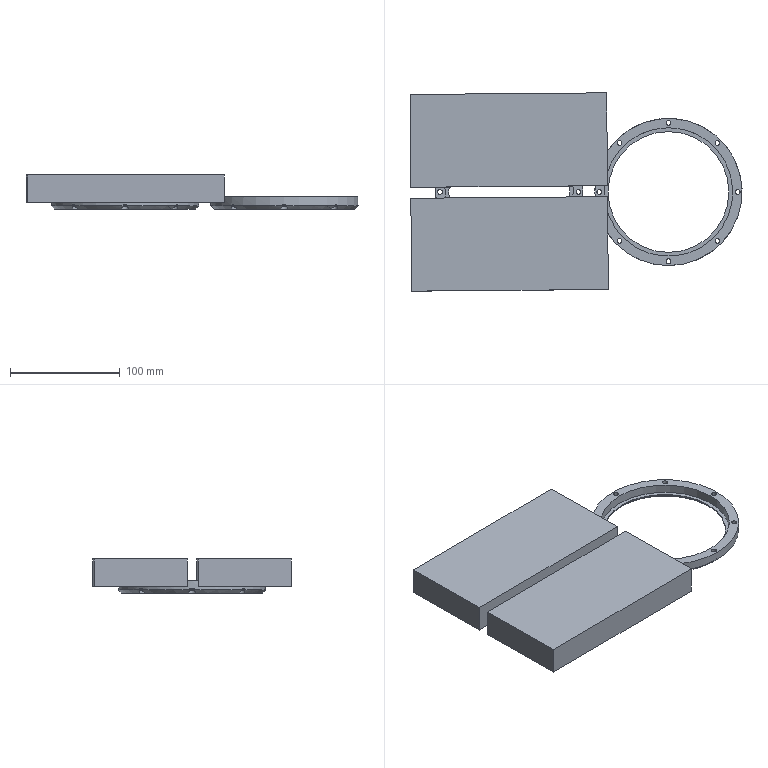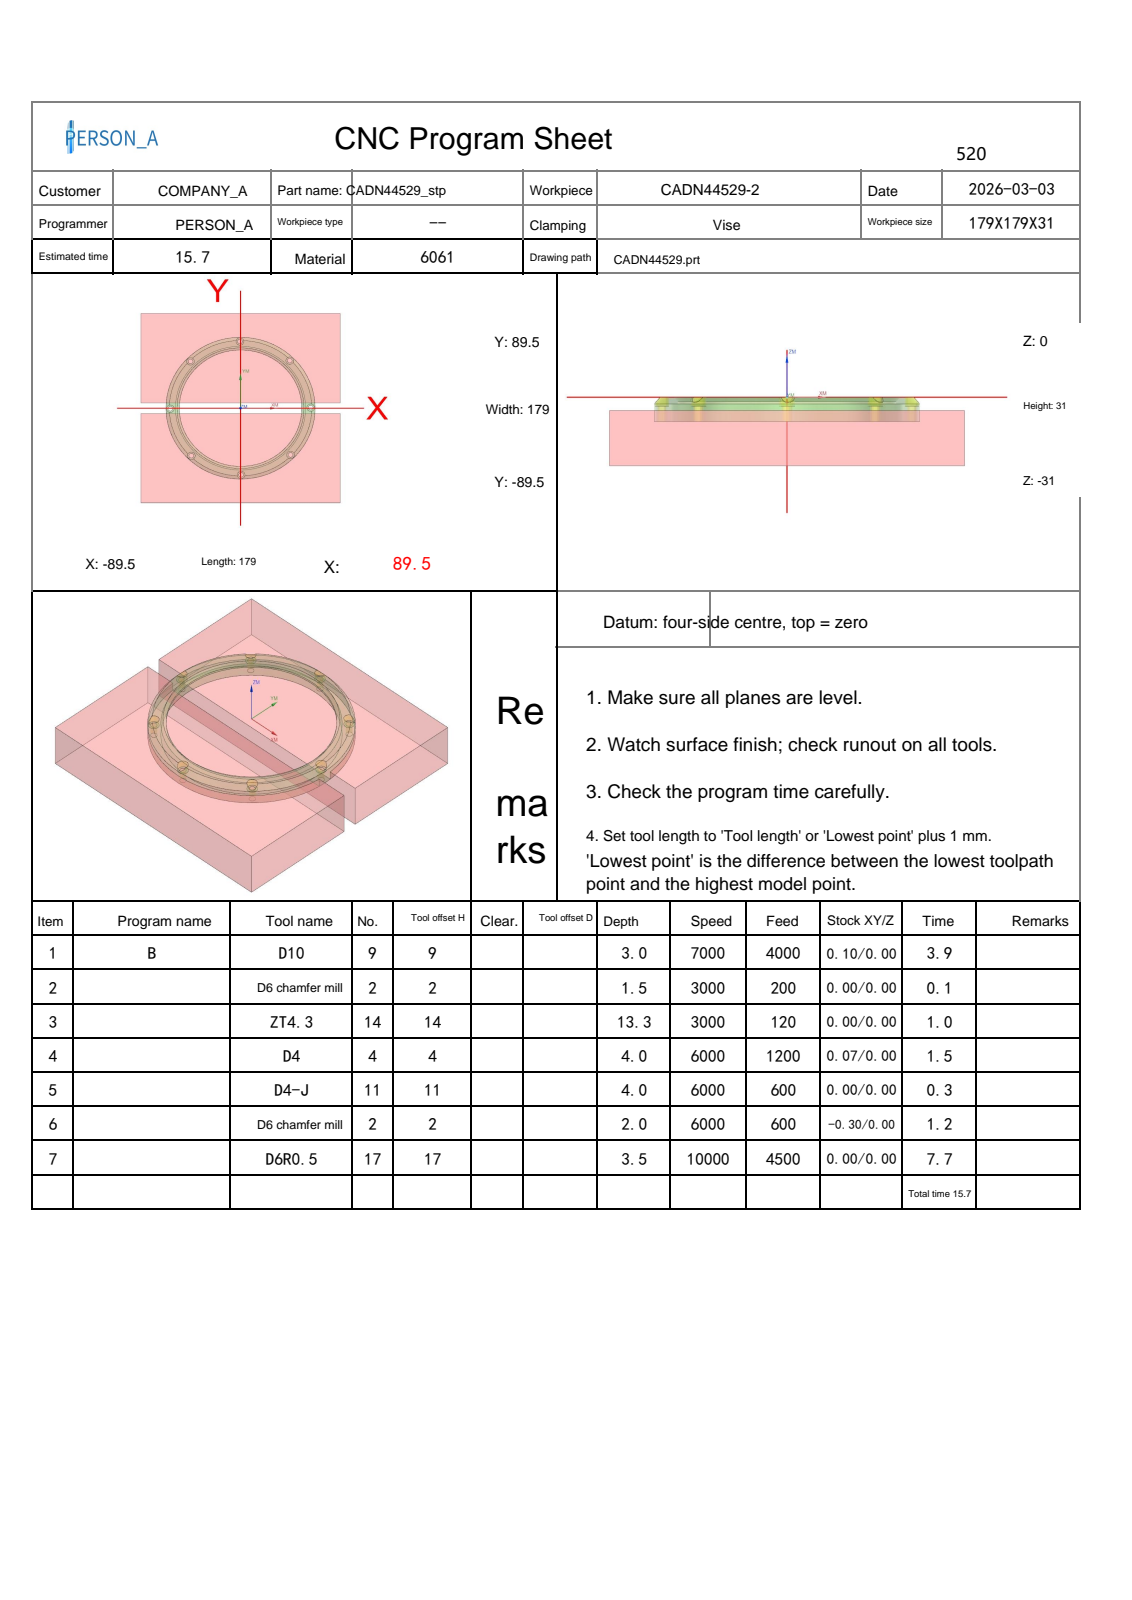NC program | NX | posted by the shop | part box 302.234 x 180.468 x 31 mm
Lines 22986 to 24363 of 75694:
N7 T17 M06
(D6R0.5  D=6. R=0.5 H=17 ce=0.00 di=0.00)
G00 G90 G54 X46.376 Y-28.084 M03 S10000
G43 H17 Z50.
M08
Z1.5
G01 X46.877 Y-27.259 Z1.449 F4500.
X47.6 Y-25.976 Z1.372
X48.553 Y-24.148 Z1.264
X49.436 Y-22.285 Z1.156
X50.247 Y-20.39 Z1.048
X50.986 Y-18.466 Z.94
X51.651 Y-16.515 Z.832
X52.241 Y-14.54 Z.724
X52.756 Y-12.544 Z.616
X53.194 Y-10.53 Z.508
X53.556 Y-8.501 Z.4
X53.84 Y-6.459 Z.292
X54.047 Y-4.408 Z.184
X54.175 Y-2.351 Z.076
X54.226 Y-.29 Z-.032
X54.22 Y.446 Z-.071
G03 X0.0 Y54.221 I-54.22 J-.447
X-54.221 Y-.001 I0.0 J-54.221
X0.0 Y-54.222 I54.221 J0.0
X54.221 Y-.001 I0.0 J54.221
X54.22 Y.446 I-54.221 J0.0
G01 X54.215 Y.814
X54.209 Y1.181
X54.198 Y1.549
X54.188 Y1.916
X54.157 Y2.651
X54.116 Y3.385
X54.064 Y4.119 Z-.072
X54.003 Y4.851
X53.933 Y5.583
X53.852 Y6.314
X53.761 Y7.044
X53.66 Y7.772
X53.55 Y8.499
X53.429 Y9.224 Z-.073
X53.299 Y9.948
X53.159 Y10.67
X53.01 Y11.389
X52.85 Y12.107
X52.681 Y12.823
X52.502 Y13.536 Z-.074
X52.313 Y14.247
X52.115 Y14.955
X51.908 Y15.66
X51.69 Y16.362
X51.463 Y17.062
X51.227 Y17.758
X50.982 Y18.451 Z-.075
X50.726 Y19.14
X50.462 Y19.826
X50.188 Y20.509
X49.906 Y21.187
X49.614 Y21.862
X49.312 Y22.533 Z-.076
X49.002 Y23.199
X48.683 Y23.862
X48.355 Y24.52
X48.018 Y25.173
X47.672 Y25.822
X47.317 Y26.466
X46.954 Y27.105 Z-.077
X46.582 Y27.739
X46.201 Y28.368
X45.812 Y28.992
X45.414 Y29.61
X45.009 Y30.223
X44.594 Y30.831 Z-.078
X44.172 Y31.433
X43.742 Y32.029
X43.303 Y32.619
X42.857 Y33.203
X42.402 Y33.781
X41.94 Y34.353
X41.471 Y34.918 Z-.079
X40.993 Y35.477
X40.508 Y36.03
X40.016 Y36.575
X39.516 Y37.115
X39.009 Y37.647
X38.495 Y38.172 Z-.08
X37.973 Y38.691
X37.445 Y39.202
X36.91 Y39.706
X36.368 Y40.203
X35.819 Y40.692
X35.264 Y41.174
X34.702 Y41.648 Z-.081
X34.134 Y42.115
X33.56 Y42.574
X32.98 Y43.025
X32.393 Y43.468
X31.8 Y43.903
X31.202 Y44.33
X30.598 Y44.749 Z-.082
X29.988 Y45.16
X29.373 Y45.562
X28.752 Y45.956
X28.127 Y46.342
X27.495 Y46.719
X26.859 Y47.087 Z-.083
X26.218 Y47.447
X25.572 Y47.798
X24.922 Y48.14
X24.267 Y48.474
X23.607 Y48.798
X22.943 Y49.114
X22.275 Y49.42 Z-.084
X21.603 Y49.717
X20.926 Y50.006
X20.246 Y50.285
X19.562 Y50.554
X18.875 Y50.815
X18.184 Y51.066 Z-.085
X17.49 Y51.308
X16.793 Y51.54
X16.092 Y51.763
X15.389 Y51.976
X14.682 Y52.18
X13.973 Y52.374
X13.262 Y52.559 Z-.086
X12.548 Y52.734
X11.832 Y52.899
X11.113 Y53.054
X10.393 Y53.2
X9.67 Y53.336
X8.946 Y53.462 Z-.087
X8.22 Y53.578
X7.493 Y53.684
X6.764 Y53.781
X6.034 Y53.868
X5.303 Y53.944
X4.571 Y54.011
X3.838 Y54.068 Z-.088
X3.105 Y54.115
X2.371 Y54.152
X1.636 Y54.179
X.901 Y54.196
X.289 Y54.201
X-.324 Y54.202
X-.446
X-.569 Y54.2 Z-.089
X-1.296 Y54.187
X-2.024 Y54.165
X-2.751 Y54.133
X-3.477 Y54.091
X-4.203 Y54.039
X-4.928 Y53.978
X-5.652 Y53.907 Z-.09
X-6.376 Y53.826
X-7.098 Y53.735
X-7.818 Y53.635
X-8.538 Y53.525
X-9.255 Y53.405
X-9.972 Y53.276
X-10.686 Y53.137 Z-.091
X-11.398 Y52.989
X-12.109 Y52.831
X-12.817 Y52.663
X-13.523 Y52.486
X-14.226 Y52.3
X-14.927 Y52.104 Z-.092
X-15.625 Y51.899
X-16.32 Y51.684
X-17.013 Y51.46
X-17.702 Y51.227
X-18.388 Y50.985
X-19.071 Y50.733
X-19.75 Y50.472 Z-.093
X-20.426 Y50.203
X-21.098 Y49.924
X-21.766 Y49.636
X-22.431 Y49.339
X-23.091 Y49.033
X-23.747 Y48.719 Z-.094
X-24.399 Y48.395
X-25.046 Y48.063
X-25.689 Y47.723
X-26.328 Y47.373
X-26.961 Y47.015
X-27.59 Y46.649
X-28.214 Y46.274 Z-.095
X-28.832 Y45.891
X-29.446 Y45.5
X-30.054 Y45.1
X-30.656 Y44.693
X-31.254 Y44.277
X-31.845 Y43.853
X-32.431 Y43.422 Z-.096
X-33.011 Y42.982
X-33.585 Y42.535
X-34.153 Y42.08
X-34.714 Y41.618
X-35.27 Y41.148
X-35.819 Y40.671 Z-.097
X-36.362 Y40.186
X-36.898 Y39.694
X-37.427 Y39.195
X-37.95 Y38.689
X-38.466 Y38.176
X-38.975 Y37.656
X-39.477 Y37.129 Z-.098
X-39.972 Y36.596
X-40.459 Y36.056
X-40.94 Y35.509
X-41.413 Y34.956
X-41.878 Y34.397
X-42.336 Y33.832
X-42.786 Y33.26 Z-.099
X-43.229 Y32.683
X-43.663 Y32.099
X-44.09 Y31.51
X-44.509 Y30.915
X-44.92 Y30.315
X-45.323 Y29.709 Z-.1
X-45.718 Y29.098
X-46.104 Y28.481
X-46.482 Y27.86
X-46.852 Y27.233
X-47.213 Y26.601
X-47.566 Y25.965
X-47.91 Y25.324 Z-.101
X-48.246 Y24.679
X-48.572 Y24.029
X-48.891 Y23.374
X-49.2 Y22.716
X-49.5 Y22.053
X-49.792 Y21.386 Z-.102
X-50.074 Y20.716
X-50.348 Y20.042
X-50.612 Y19.364
X-50.867 Y18.683
X-51.113 Y17.998
X-51.35 Y17.31
X-51.578 Y16.619 Z-.103
X-51.796 Y15.925
X-52.005 Y15.228
X-52.205 Y14.529
X-52.395 Y13.827
X-52.576 Y13.122
X-52.747 Y12.415
X-52.909 Y11.706 Z-.104
X-53.061 Y10.994
X-53.204 Y10.281
X-53.337 Y9.566
X-53.46 Y8.849
X-53.574 Y8.13
X-53.678 Y7.41 Z-.105
X-53.773 Y6.689
X-53.858 Y5.966
X-53.933 Y5.243
X-53.998 Y4.518
X-54.054 Y3.793
X-54.1 Y3.067
X-54.136 Y2.34 Z-.106
X-54.162 Y1.613
X-54.179 Y.886
X-54.186 Y.158
X-54.183 Y-.569
X-54.17 Y-1.296
X-54.148 Y-2.024 Z-.107
X-54.116 Y-2.75
X-54.074 Y-3.477
X-54.022 Y-4.202
X-53.961 Y-4.927
X-53.89 Y-5.651
X-53.809 Y-6.374
X-53.718 Y-7.096 Z-.108
X-53.618 Y-7.816
X-53.508 Y-8.535
X-53.388 Y-9.253
X-53.259 Y-9.969
X-53.121 Y-10.683
X-52.972 Y-11.395
X-52.814 Y-12.105 Z-.109
X-52.647 Y-12.813
X-52.47 Y-13.519
X-52.284 Y-14.222
X-52.088 Y-14.923
X-51.883 Y-15.62
X-51.668 Y-16.316 Z-.11
X-51.444 Y-17.008
X-51.211 Y-17.697
X-50.969 Y-18.383
X-50.717 Y-19.065
X-50.457 Y-19.744
X-50.187 Y-20.42
X-49.908 Y-21.092 Z-.111
X-49.621 Y-21.76
X-49.324 Y-22.424
X-49.018 Y-23.084
X-48.704 Y-23.74
X-48.381 Y-24.392
X-48.049 Y-25.039
X-47.708 Y-25.682 Z-.112
X-47.359 Y-26.32
X-47.061 Y-26.847
X-46.758 Y-27.37
X-46.696 Y-27.476
X-46.635 Y-27.582
X-46.26 Y-28.205
X-45.877 Y-28.824
X-45.486 Y-29.437 Z-.113
X-45.087 Y-30.045
X-44.679 Y-30.647
X-44.263 Y-31.244
X-43.84 Y-31.835
X-43.408 Y-32.421
X-42.969 Y-33.001
X-42.522 Y-33.575 Z-.114
X-42.067 Y-34.142
X-41.605 Y-34.704
X-41.135 Y-35.259
X-40.658 Y-35.808
X-40.174 Y-36.351
X-39.682 Y-36.887 Z-.115
X-39.183 Y-37.416
X-38.677 Y-37.938
X-38.164 Y-38.454
X-37.644 Y-38.963
X-37.118 Y-39.465
X-36.584 Y-39.959
X-36.044 Y-40.447 Z-.116
X-35.498 Y-40.927
X-34.945 Y-41.4
X-34.386 Y-41.865
X-33.821 Y-42.323
X-33.25 Y-42.773
X-32.672 Y-43.215
X-32.089 Y-43.65 Z-.117
X-31.5 Y-44.076
X-30.906 Y-44.495
X-30.305 Y-44.906
X-29.7 Y-45.309
X-29.089 Y-45.703
X-28.472 Y-46.089 Z-.118
X-27.851 Y-46.467
X-27.224 Y-46.837
X-26.593 Y-47.198
X-25.957 Y-47.551
X-25.316 Y-47.895
X-24.671 Y-48.23
X-24.021 Y-48.557 Z-.119
X-23.367 Y-48.875
X-22.709 Y-49.184
X-22.046 Y-49.484
X-21.38 Y-49.776
X-20.71 Y-50.058
X-20.036 Y-50.331
X-19.358 Y-50.596 Z-.12
X-18.677 Y-50.851
X-17.993 Y-51.097
X-17.305 Y-51.334
X-16.614 Y-51.561
X-15.92 Y-51.779
X-15.224 Y-51.988 Z-.121
X-14.525 Y-52.188
X-13.823 Y-52.378
X-13.118 Y-52.559
X-12.411 Y-52.73
X-11.702 Y-52.892
X-10.991 Y-53.044
X-10.278 Y-53.186 Z-.122
X-9.563 Y-53.319
X-8.846 Y-53.443
X-8.128 Y-53.557
X-7.408 Y-53.661
X-6.687 Y-53.755
X-5.965 Y-53.84 Z-.123
X-5.241 Y-53.915
X-4.879 Y-53.949
X-4.517 Y-53.981
X-4.155 Y-54.01
X-3.792 Y-54.036
X-3.429 Y-54.061
X-3.066 Y-54.082
X-2.703 Y-54.102
X-2.34 Y-54.118
X-1.977 Y-54.133
X-1.613 Y-54.145
X-1.25 Y-54.154
X-.886 Y-54.161 Z-.124
X-.159 Y-54.168
X.568 Y-54.166
X1.295 Y-54.152
X2.022 Y-54.13
X2.386 Y-54.116
X2.749 Y-54.098
X3.112 Y-54.079
X3.475 Y-54.056
X3.838 Y-54.032 Z-.125
X4.2 Y-54.004
X4.563 Y-53.975
X4.925 Y-53.943
X5.287 Y-53.909
X5.649 Y-53.872
X6.01 Y-53.833
X6.371 Y-53.791
X6.732 Y-53.747
X7.093 Y-53.7
X7.453 Y-53.652
X7.813 Y-53.6
X8.173 Y-53.547
X8.532 Y-53.49 Z-.126
X8.891 Y-53.432
X9.249 Y-53.371
X9.607 Y-53.308
X9.965 Y-53.242
X10.322 Y-53.174
X10.679 Y-53.103
X11.035 Y-53.031
X11.391 Y-52.955
X11.746 Y-52.878
X12.101 Y-52.797
X12.455 Y-52.715
X12.808 Y-52.629
X13.161 Y-52.543 Z-.127
X13.514 Y-52.452
X13.866 Y-52.361
X14.216 Y-52.266
X14.567 Y-52.17
X14.917 Y-52.07
X15.266 Y-51.97
X15.615 Y-51.865
X15.963 Y-51.76
X16.309 Y-51.651
X16.656 Y-51.541
X17.001 Y-51.427
X17.346 Y-51.313
X17.69 Y-51.194
X18.034 Y-51.075 Z-.128
X18.376 Y-50.952
X18.718 Y-50.828
X19.058 Y-50.7
X19.398 Y-50.572
X19.737 Y-50.44
X20.075 Y-50.307
X20.412 Y-50.17
X20.749 Y-50.033
X21.084 Y-49.892
X21.419 Y-49.75
X21.752 Y-49.604
X22.085 Y-49.458
X22.416 Y-49.307 Z-.129
X22.746 Y-49.156
X23.075 Y-49.002
X23.404 Y-48.847
X23.731 Y-48.687
X24.058 Y-48.528
X24.383 Y-48.364
X24.707 Y-48.2
X25.03 Y-48.033
X25.352 Y-47.864
X25.672 Y-47.692
X26.31 Y-47.343
X26.943 Y-46.985 Z-.13
X27.572 Y-46.619
X28.195 Y-46.245
X28.813 Y-45.862
X29.426 Y-45.471
X30.034 Y-45.072
X30.636 Y-44.664 Z-.131
X31.233 Y-44.249
X31.824 Y-43.825
X32.409 Y-43.394
X32.989 Y-42.955
X33.563 Y-42.508
X34.13 Y-42.053
X34.692 Y-41.591 Z-.132
X35.247 Y-41.122
X35.795 Y-40.645
X36.338 Y-40.16
X36.874 Y-39.669
X37.403 Y-39.17
X37.925 Y-38.664
X38.441 Y-38.152 Z-.133
X38.949 Y-37.632
X39.451 Y-37.106
X39.945 Y-36.573
X40.433 Y-36.033
X40.913 Y-35.487
X41.385 Y-34.934 Z-.134
X41.85 Y-34.375
X42.308 Y-33.81
X42.758 Y-33.239
X43.2 Y-32.662
X43.635 Y-32.079
X44.061 Y-31.49
X44.48 Y-30.896 Z-.135
X44.891 Y-30.296
X45.293 Y-29.69
X45.688 Y-29.08
X46.074 Y-28.464
X46.452 Y-27.842
X46.76 Y-27.322
X47.063 Y-26.798 Z-.136
X47.122 Y-26.692
X47.182 Y-26.585
X47.525 Y-25.968
X47.859 Y-25.346
X48.185 Y-24.72
X48.503 Y-24.09
X48.813 Y-23.456
X49.114 Y-22.818 Z-.137
X49.408 Y-22.176
X49.692 Y-21.53
X49.969 Y-20.88
X50.237 Y-20.227
X50.496 Y-19.571
X50.746 Y-18.911
X50.988 Y-18.248 Z-.138
X51.221 Y-17.582
X51.446 Y-16.912
X51.662 Y-16.24
X51.869 Y-15.566
X52.067 Y-14.888
X52.257 Y-14.208
X52.437 Y-13.526 Z-.139
X52.609 Y-12.841
X52.772 Y-12.155
X52.925 Y-11.466
X53.07 Y-10.775
X53.206 Y-10.082
X53.333 Y-9.388
X53.45 Y-8.692 Z-.14
X53.559 Y-7.995
X53.659 Y-7.296
X53.749 Y-6.596
X53.83 Y-5.895
X53.902 Y-5.193
X53.966 Y-4.49
X54.019 Y-3.786 Z-.141
X54.064 Y-3.082
X54.1 Y-2.377
X54.126 Y-1.672
X54.143 Y-.966
X54.151 Y-.26
X54.149 Y.446 Z-.142
X54.145 Y.812
X54.138 Y1.178
X54.129 Y1.544
X54.117 Y1.91
X54.087 Y2.641
X54.046 Y3.372
X53.995 Y4.103
X53.934 Y4.832
X53.864 Y5.561 Z-.143
X53.784 Y6.289
X53.694 Y7.016
X53.594 Y7.741
X53.484 Y8.465
X53.364 Y9.187
X53.235 Y9.908
X53.096 Y10.627 Z-.144
X52.948 Y11.344
X52.789 Y12.059
X52.621 Y12.771
X52.443 Y13.482
X52.256 Y14.189
X52.059 Y14.895 Z-.145
X51.853 Y15.597
X51.637 Y16.297
X51.412 Y16.994
X51.177 Y17.687
X50.934 Y18.377
X50.68 Y19.064
X50.418 Y19.748 Z-.146
X50.146 Y20.428
X50.006 Y20.766
X49.865 Y21.104
X49.721 Y21.44
X49.575 Y21.776
X49.426 Y22.111
X49.276 Y22.444
X49.122 Y22.777
X48.968 Y23.109
X48.81 Y23.439
X48.651 Y23.769 Z-.147
X48.488 Y24.097
X48.325 Y24.424
X48.158 Y24.75
X47.99 Y25.075
X47.819 Y25.399
X47.646 Y25.722
X47.471 Y26.043
X47.294 Y26.364
X47.114 Y26.683
X46.933 Y27.001
X46.749 Y27.317
X46.563 Y27.633
X46.375 Y27.947 Z-.148
X46.185 Y28.26
X45.988 Y28.578
X45.79 Y28.895
X45.598 Y29.197
X45.404 Y29.498
X45.203 Y29.804
X45.001 Y30.109
X44.796 Y30.413
X44.59 Y30.715
X44.381 Y31.015
X44.17 Y31.315
X43.957 Y31.613
X43.742 Y31.909 Z-.149
X43.525 Y32.204
X43.307 Y32.498
X43.086 Y32.789
X42.863 Y33.08
X42.639 Y33.369
X42.412 Y33.657
X42.183 Y33.942
X41.953 Y34.227
X41.72 Y34.51
X41.486 Y34.791
X41.25 Y35.07
X41.012 Y35.349
X40.772 Y35.625 Z-.15
X40.53 Y35.9
X40.286 Y36.173
X40.041 Y36.444
X39.793 Y36.714
X39.544 Y36.982
X39.293 Y37.249
X39.04 Y37.514
X38.786 Y37.777
X38.53 Y38.038
X38.271 Y38.297
X38.012 Y38.555
X37.75 Y38.811
X37.487 Y39.066 Z-.151
X37.222 Y39.318
X36.955 Y39.569
X36.686 Y39.818
X36.416 Y40.065
X36.145 Y40.31
X35.871 Y40.553
X35.596 Y40.795
X35.32 Y41.035
X35.041 Y41.272
X34.761 Y41.508
X34.48 Y41.742
X34.197 Y41.975
X33.912 Y42.205
X33.626 Y42.433 Z-.152
X33.338 Y42.659
X33.049 Y42.884
X32.758 Y43.106
X32.466 Y43.326
X32.172 Y43.545
X31.877 Y43.761
X31.581 Y43.976
X31.282 Y44.188
X30.983 Y44.399
X30.682 Y44.607
X30.38 Y44.813
X30.076 Y45.018
X29.771 Y45.22 Z-.153
X29.464 Y45.42
X29.157 Y45.618
X28.847 Y45.814
X28.537 Y46.008
X28.225 Y46.2
X27.912 Y46.39
X27.598 Y46.577
X27.282 Y46.763
X26.966 Y46.946
X26.648 Y47.127
X26.328 Y47.306
X26.008 Y47.483
X25.686 Y47.658 Z-.154
X25.363 Y47.83
X25.039 Y48.001
X24.714 Y48.169
X24.388 Y48.335
X24.061 Y48.498
X23.732 Y48.66
X23.402 Y48.819
X23.072 Y48.976
X22.74 Y49.131
X22.407 Y49.284
X22.074 Y49.434
X21.739 Y49.582
X21.403 Y49.728 Z-.155
X21.066 Y49.871
X20.729 Y50.012
X20.39 Y50.151
X20.051 Y50.288
X19.71 Y50.422
X19.369 Y50.554
X19.026 Y50.684
X18.683 Y50.812
X18.339 Y50.937
X17.994 Y51.059
X17.649 Y51.18
X17.302 Y51.298
X16.955 Y51.414 Z-.156
X16.607 Y51.527
X16.258 Y51.638
X15.909 Y51.747
X15.559 Y51.853
X15.208 Y51.957
X14.856 Y52.059
X14.504 Y52.158
X14.151 Y52.254
X13.797 Y52.349
X13.443 Y52.441
X13.088 Y52.531
X12.732 Y52.618
X12.376 Y52.703 Z-.157
X12.02 Y52.785
X11.663 Y52.865
X11.305 Y52.942
X10.947 Y53.018
X10.588 Y53.09
X10.229 Y53.161
X9.869 Y53.228
X9.509 Y53.294
X9.148 Y53.357
X8.788 Y53.418
X8.426 Y53.476
X8.064 Y53.531
X7.702 Y53.585 Z-.158
X7.34 Y53.635
X6.977 Y53.684
X6.614 Y53.73
X6.25 Y53.773
X5.887 Y53.814
X5.523 Y53.852
X5.159 Y53.889
X4.794 Y53.922
X4.429 Y53.953
X4.064 Y53.982
X3.699 Y54.008
X3.334 Y54.032
X2.969 Y54.053
X2.603 Y54.071 Z-.159
X2.238 Y54.088
X1.872 Y54.102
X1.506 Y54.113
X1.14 Y54.122
X.408 Y54.132
X-.324 Y54.133
X-1.05 Y54.122
X-1.777 Y54.104
X-2.503 Y54.075 Z-.16
X-3.229 Y54.037
X-3.954 Y53.988
X-4.678 Y53.93
X-5.402 Y53.862
X-6.125 Y53.785
X-6.846 Y53.698 Z-.161
X-7.566 Y53.601
X-8.285 Y53.494
X-9.003 Y53.378
X-9.719 Y53.252
X-10.433 Y53.117
X-11.145 Y52.972
X-11.855 Y52.817 Z-.162
X-12.563 Y52.653
X-13.269 Y52.48
X-13.972 Y52.297
X-14.673 Y52.104
X-15.371 Y51.902
X-16.066 Y51.691 Z-.163
X-16.759 Y51.471
X-17.448 Y51.241
X-18.134 Y51.002
X-18.817 Y50.754
X-19.497 Y50.496
X-20.173 Y50.23
X-20.846 Y49.954 Z-.164
X-21.514 Y49.67
X-22.179 Y49.377
X-22.84 Y49.074
X-23.497 Y48.763
X-24.149 Y48.443
X-24.797 Y48.114
X-25.441 Y47.777 Z-.165
X-26.08 Y47.431
X-26.714 Y47.076
X-27.344 Y46.713
X-27.969 Y46.342
X-28.588 Y45.962
X-29.203 Y45.574 Z-.166
X-29.812 Y45.178
X-30.415 Y44.773
X-31.014 Y44.361
X-31.606 Y43.94
X-32.193 Y43.512
X-32.775 Y43.076
X-33.35 Y42.632 Z-.167
X-33.919 Y42.18
X-34.482 Y41.721
X-35.039 Y41.254
X-35.59 Y40.78
X-36.134 Y40.298
X-36.671 Y39.809
X-37.203 Y39.313 Z-.168
X-37.727 Y38.81
X-38.244 Y38.3
X-38.755 Y37.783
X-39.259 Y37.259
X-39.755 Y36.729
X-40.245 Y36.192 Z-.169
X-40.727 Y35.648
X-41.202 Y35.098
X-41.669 Y34.541
X-42.129 Y33.979
X-42.581 Y33.41
X-43.026 Y32.835
X-43.462 Y32.255 Z-.17
X-43.891 Y31.668
X-44.312 Y31.076
X-44.726 Y30.478
X-45.131 Y29.875
X-45.527 Y29.266
X-45.822 Y28.802
X-46.113 Y28.335 Z-.171
X-46.205 Y28.184
X-46.297 Y28.033
X-46.669 Y27.409
X-47.032 Y26.78
X-47.387 Y26.146
X-47.734 Y25.507
X-48.072 Y24.864
X-48.401 Y24.216 Z-.172
X-48.722 Y23.564
X-49.034 Y22.908
X-49.337 Y22.248
X-49.631 Y21.583
X-49.916 Y20.915
X-50.192 Y20.243
X-50.459 Y19.567 Z-.173
X-50.717 Y18.888
X-50.966 Y18.205
X-51.206 Y17.519
X-51.436 Y16.83
X-51.657 Y16.138
X-51.869 Y15.443 Z-.174
X-52.072 Y14.745
X-52.265 Y14.045
X-52.449 Y13.342
X-52.623 Y12.637
X-52.788 Y11.929
X-52.943 Y11.219
X-53.089 Y10.507 Z-.175
X-53.225 Y9.794
X-53.351 Y9.078
X-53.468 Y8.361
X-53.575 Y7.642
X-53.673 Y6.923
X-53.761 Y6.201
X-53.839 Y5.479 Z-.176
X-53.908 Y4.756
X-53.967 Y4.031
X-54.016 Y3.307
X-54.055 Y2.581
X-54.085 Y1.855
X-54.105 Y1.129 Z-.177
X-54.115 Y.402
Y-.324
X-54.106 Y-1.051
X-54.087 Y-1.777
X-54.058 Y-2.503
X-54.019 Y-3.228
X-53.971 Y-3.953 Z-.178
X-53.913 Y-4.677
X-53.845 Y-5.401
X-53.767 Y-6.123
X-53.68 Y-6.844
X-53.583 Y-7.564
X-53.477 Y-8.283 Z-.179
X-53.361 Y-9.
X-53.235 Y-9.716
X-53.099 Y-10.43
X-52.954 Y-11.141
X-52.8 Y-11.851
X-52.636 Y-12.559
X-52.462 Y-13.265 Z-.18
X-52.28 Y-13.968
X-52.087 Y-14.668
X-51.885 Y-15.366
X-51.674 Y-16.061
X-51.454 Y-16.754
X-51.224 Y-17.443
X-50.985 Y-18.129 Z-.181
X-50.737 Y-18.812
X-50.48 Y-19.491
X-50.213 Y-20.167
X-49.938 Y-20.839
X-49.654 Y-21.508
X-49.36 Y-22.172 Z-.182
X-49.058 Y-22.833
X-48.747 Y-23.489
X-48.427 Y-24.142
X-48.098 Y-24.79
X-47.761 Y-25.433
X-47.415 Y-26.072
X-47.061 Y-26.706 Z-.183
X-46.698 Y-27.335
X-46.327 Y-27.96
X-45.947 Y-28.579
X-45.559 Y-29.193
X-45.163 Y-29.802
X-44.759 Y-30.406 Z-.184
X-44.346 Y-31.004
X-43.926 Y-31.596
X-43.498 Y-32.183
X-43.062 Y-32.764
X-42.618 Y-33.339
X-42.166 Y-33.908
X-41.707 Y-34.471 Z-.185
X-41.24 Y-35.028
X-40.766 Y-35.578
X-40.285 Y-36.122
X-39.796 Y-36.66
X-39.3 Y-37.19
X-38.797 Y-37.715
X-38.287 Y-38.232 Z-.186
X-37.771 Y-38.742
X-37.247 Y-39.246
X-36.717 Y-39.742
X-36.18 Y-40.231
X-35.636 Y-40.713
X-35.086 Y-41.188 Z-.187
X-34.53 Y-41.655
X-33.968 Y-42.115
X-33.399 Y-42.567
X-32.825 Y-43.012
X-32.244 Y-43.448
X-31.658 Y-43.877
X-31.066 Y-44.298 Z-.188
X-30.468 Y-44.711
X-29.865 Y-45.116
X-29.257 Y-45.513
X-28.643 Y-45.901
X-28.024 Y-46.281
X-27.4 Y-46.653
X-26.771 Y-47.017 Z-.189
X-26.138 Y-47.372
X-25.499 Y-47.718
X-24.856 Y-48.056
X-24.209 Y-48.385
X-23.557 Y-48.706
X-22.901 Y-49.018 Z-.19
X-22.241 Y-49.321
X-21.576 Y-49.615
X-20.908 Y-49.9
X-20.237 Y-50.176
X-19.561 Y-50.443
X-18.882 Y-50.701
X-18.2 Y-50.949 Z-.191
X-17.514 Y-51.189
X-16.825 Y-51.419
X-16.133 Y-51.64
X-15.438 Y-51.852
X-14.741 Y-52.055
X-14.041 Y-52.248 Z-.192
X-13.338 Y-52.431
X-12.633 Y-52.606
X-11.925 Y-52.77
X-11.216 Y-52.926
X-10.504 Y-53.071
X-9.791 Y-53.207
X-9.076 Y-53.334 Z-.193
X-8.359 Y-53.451
X-7.64 Y-53.558
X-6.921 Y-53.655
X-6.583 Y-53.698
X-6.244 Y-53.738
X-5.861 Y-53.781
X-5.478 Y-53.822
X-4.755 Y-53.89
X-4.031 Y-53.949 Z-.194
X-3.306 Y-53.998
X-2.581 Y-54.037
X-1.855 Y-54.067
X-1.129 Y-54.087
X-.403 Y-54.097
X.324 Z-.195
X1.05 Y-54.088
X1.776 Y-54.069
X2.501 Y-54.04
X3.227 Y-54.002
X3.951 Y-53.953
X4.675 Y-53.895
X5.189 Y-53.848 Z-.196
X5.702 Y-53.796
X5.911 Y-53.773
X6.121 Y-53.75
X6.842 Y-53.663
X7.561 Y-53.566
X8.28 Y-53.459
X8.997 Y-53.343
X9.712 Y-53.218
X10.426 Y-53.082 Z-.197
X11.137 Y-52.937
X11.847 Y-52.783
X12.554 Y-52.619
X13.26 Y-52.445
X13.963 Y-52.263
X14.663 Y-52.07 Z-.198
X15.361 Y-51.869
X16.055 Y-51.658
X16.748 Y-51.437
X17.436 Y-51.208
X18.122 Y-50.969
X18.805 Y-50.721
X19.484 Y-50.464 Z-.199
X20.16 Y-50.197
X20.832 Y-49.922
X21.5 Y-49.638
X22.164 Y-49.344
X22.825 Y-49.042
X23.481 Y-48.731 Z-.2
X24.133 Y-48.412
X24.781 Y-48.083
X25.424 Y-47.746
X26.063 Y-47.4
X26.697 Y-47.046
X27.326 Y-46.683
X27.95 Y-46.312 Z-.201
X28.569 Y-45.932
X29.183 Y-45.545
X29.792 Y-45.149
X30.395 Y-44.744
X30.993 Y-44.332
X31.585 Y-43.912
X32.172 Y-43.484 Z-.202
X32.753 Y-43.048
X33.328 Y-42.604
X33.896 Y-42.153
X34.459 Y-41.694
X35.016 Y-41.227
X35.566 Y-40.753 Z-.203
X36.11 Y-40.272
X36.647 Y-39.784
X37.178 Y-39.288
X37.702 Y-38.785
X38.219 Y-38.275
X38.729 Y-37.759
X39.233 Y-37.235 Z-.204
X39.729 Y-36.705
X40.218 Y-36.168
X40.7 Y-35.625
X41.174 Y-35.075
X41.641 Y-34.519
X42.101 Y-33.957 Z-.205
X42.553 Y-33.389
X42.997 Y-32.814
X43.434 Y-32.234
X43.862 Y-31.648
X44.283 Y-31.056
X44.696 Y-30.459
X45.101 Y-29.856 Z-.206
X45.497 Y-29.248
X45.886 Y-28.634
X46.266 Y-28.015
X46.638 Y-27.392
X47.001 Y-26.763
X47.349 Y-26.143
X47.688 Y-25.518 Z-.207
X48.019 Y-24.889
X48.342 Y-24.255
X48.657 Y-23.618
X48.963 Y-22.976
X49.261 Y-22.33
X49.55 Y-21.681
X49.83 Y-21.027 Z-.208
X50.102 Y-20.37
X50.366 Y-19.71
X50.62 Y-19.046
X50.866 Y-18.379
X51.103 Y-17.709
X51.332 Y-17.035 Z-.209
X51.551 Y-16.359
X51.761 Y-15.68
X51.963 Y-14.998
X52.155 Y-14.314
X52.339 Y-13.627
X52.513 Y-12.937
X52.679 Y-12.246 Z-.21
X52.835 Y-11.552
X52.982 Y-10.857
X53.12 Y-10.159
X53.249 Y-9.46
X53.369 Y-8.759
X53.479 Y-8.057
X53.58 Y-7.353 Z-.211
X53.672 Y-6.648
X53.755 Y-5.942
X53.828 Y-5.235
X53.892 Y-4.527
X53.947 Y-3.818
X53.992 Y-3.108
X54.028 Y-2.398 Z-.212
X54.055 Y-1.688
X54.072 Y-.977
X54.08 Y-.266
X54.079 Y.445
X54.068 Y1.159
X54.048 Y1.873 Z-.213
X54.018 Y2.587
X53.979 Y3.3
X53.931 Y4.012
X53.873 Y4.724
X53.806 Y5.435
X53.729 Y6.146
X53.643 Y6.855 Z-.214
X53.548 Y7.562
X53.443 Y8.269
X53.329 Y8.974
X53.206 Y9.678
X53.073 Y10.379
X52.931 Y11.079
X52.78 Y11.777 Z-.215
X52.62 Y12.473
X52.451 Y13.167
X52.272 Y13.859
X52.084 Y14.548
X51.887 Y15.234
X51.682 Y15.918 Z-.216
X51.467 Y16.599
X51.243 Y17.278
X51.01 Y17.953
X50.768 Y18.625
X50.518 Y19.294
X50.258 Y19.959
X49.99 Y20.621 Z-.217
X49.714 Y21.279
X49.428 Y21.934
X49.134 Y22.585
X48.831 Y23.232
X48.52 Y23.875
X48.2 Y24.513
X47.872 Y25.148 Z-.218
X47.536 Y25.778
X47.191 Y26.403
X46.838 Y27.024
X46.477 Y27.64
X46.108 Y28.251
X45.731 Y28.858
X45.719 Y28.876
X45.707 Y28.895
X45.324 Y29.492 Z-.219
X44.933 Y30.083
X44.523 Y30.688
X44.104 Y31.287
X43.677 Y31.88
X43.241 Y32.467
X42.799 Y33.049 Z-.22
X42.348 Y33.624
X41.889 Y34.193
X41.423 Y34.756
X40.949 Y35.313
X40.468 Y35.863
X39.98 Y36.407
X39.484 Y36.944 Z-.221
X38.981 Y37.474
X38.47 Y37.998
X37.953 Y38.514
X37.429 Y39.023
X36.898 Y39.526
X36.36 Y40.021 Z-.222
X35.816 Y40.508
X35.265 Y40.989
X34.707 Y41.462
X34.144 Y41.927
X33.574 Y42.384
X32.998 Y42.834
X32.416 Y43.276 Z-.223
X31.828 Y43.71
X31.234 Y44.136
X30.634 Y44.555
X30.029 Y44.964
X29.418 Y45.366
X28.802 Y45.759
X28.181 Y46.145 Z-.224
X27.555 Y46.521
X26.923 Y46.889
X26.287 Y47.249
X25.646 Y47.6
X25. Y47.942
X24.35 Y48.275 Z-.225
X23.695 Y48.6
X23.036 Y48.915
X22.372 Y49.222
X21.705 Y49.52
X21.033 Y49.809
X20.358 Y50.088
X19.679 Y50.359 Z-.226
X18.996 Y50.62
X18.31 Y50.872
X17.621 Y51.115
X16.928 Y51.348
X16.233 Y51.572
X15.534 Y51.787 Z-.227
X14.833 Y51.992
X14.128 Y52.188
X13.422 Y52.374
X12.712 Y52.55
X12.001 Y52.717
X11.287 Y52.874
X10.571 Y53.022 Z-.228
X9.854 Y53.16
X9.134 Y53.288
X8.413 Y53.406
X7.69 Y53.515
X6.966 Y53.614
X6.241 Y53.703 Z-.229
X5.514 Y53.782
X4.787 Y53.852
X4.058 Y53.911
X3.329 Y53.961
X2.6 Y54.001
X1.869 Y54.031
X1.139 Y54.051 Z-.23
X.408 Y54.062
X-.323
X-1.053 Y54.053
X-1.784 Y54.033
X-2.514 Y54.004
X-3.244 Y53.965
X-3.973 Y53.916 Z-.231
X-4.702 Y53.857
X-5.429 Y53.789
X-6.156 Y53.71
X-6.881 Y53.622
X-7.605 Y53.524
X-8.328 Y53.416 Z-.232
X-9.049 Y53.299
X-9.769 Y53.171
X-10.487 Y53.034
X-11.203 Y52.887
X-11.917 Y52.731
X-12.628 Y52.565
X-13.338 Y52.389 Z-.233
X-14.044 Y52.204
X-14.749 Y52.009
X-15.45 Y51.805
X-16.149 Y51.591
X-16.845 Y51.368
X-17.538 Y51.136 Z-.234
X-18.227 Y50.894
X-18.914 Y50.643
X-19.596 Y50.382
X-20.276 Y50.112
X-20.951 Y49.834
X-21.623 Y49.546
X-22.29 Y49.249 Z-.235
X-22.954 Y48.943
X-23.613 Y48.628
X-24.269 Y48.304
X-24.919 Y47.972
X-25.565 Y47.63
X-26.207 Y47.28 Z-.236
X-26.843 Y46.922
X-27.475 Y46.554
X-28.102 Y46.178
X-28.723 Y45.794
X-29.34 Y45.402
X-29.951 Y45.001
X-30.556 Y44.592 Z-.237
X-31.156 Y44.174
X-31.75 Y43.749
X-32.339 Y43.316
X-32.921 Y42.875
X-33.497 Y42.426
X-34.068 Y41.969
X-34.632 Y41.504 Z-.238
X-35.19 Y41.032
X-35.741 Y40.553
X-36.286 Y40.066
X-36.824 Y39.572
X-37.355 Y39.07
X-37.88 Y38.561 Z-.239
X-38.398 Y38.046
X-38.908 Y37.523
X-39.412 Y36.994
X-39.908 Y36.457
X-40.397 Y35.915
X-40.879 Y35.365
X-41.353 Y34.809 Z-.24
X-41.82 Y34.247
X-42.279 Y33.678
X-42.73 Y33.104
X-43.173 Y32.523
X-43.609 Y31.936
X-44.037 Y31.344 Z-.241
X-44.456 Y30.746
X-44.868 Y30.142
X-45.271 Y29.533
X-45.666 Y28.918
X-46.052 Y28.298
X-46.105 Y28.212
X-46.157 Y28.126
X-46.483 Y27.584
X-46.802 Y27.039 Z-.242
X-47.164 Y26.402
X-47.518 Y25.76
X-47.862 Y25.114
X-48.198 Y24.463
X-48.525 Y23.807
X-48.843 Y23.147 Z-.243
X-49.152 Y22.483
X-49.452 Y21.814
X-49.743 Y21.142
X-50.025 Y20.466
X-50.298 Y19.786
X-50.561 Y19.102
X-50.816 Y18.415 Z-.244
X-51.06 Y17.725
X-51.296 Y17.031
X-51.522 Y16.334
X-51.738 Y15.634
X-51.945 Y14.931
X-52.143 Y14.226 Z-.245
X-52.331 Y13.518
X-52.509 Y12.807
X-52.678 Y12.094
X-52.836 Y11.379
X-52.986 Y10.662
X-53.125 Y9.943
X-53.255 Y9.222 Z-.246
X-53.375 Y8.499
X-53.485 Y7.775
X-53.585 Y7.049
X-53.676 Y6.322
X-53.756 Y5.594
X-53.827 Y4.865
X-53.888 Y4.135 Z-.247
X-53.939 Y3.404
X-53.98 Y2.672
X-54.011 Y1.94
X-54.032 Y1.208
X-54.043 Y.476
X-54.045 Y-.257 Z-.248
X-54.036 Y-.989
X-54.018 Y-1.722
X-53.989 Y-2.454
X-53.951 Y-3.185
X-53.903 Y-3.916
X-53.844 Y-4.647
X-53.776 Y-5.376 Z-.249
X-53.698 Y-6.104
X-53.611 Y-6.832
X-53.513 Y-7.558
X-53.405 Y-8.282
X-53.288 Y-9.005
X-53.161 Y-9.727 Z-.25
X-53.024 Y-10.446
X-52.877 Y-11.164
X-52.721 Y-11.88
X-52.555 Y-12.593
X-52.379 Y-13.304
X-52.194 Y-14.013
X-51.999 Y-14.719 Z-.251
X-51.795 Y-15.423
X-51.581 Y-16.123
X-51.357 Y-16.821
X-51.125 Y-17.515
X-50.882 Y-18.207
X-50.631 Y-18.895 Z-.252
X-50.37 Y-19.579
X-50.1 Y-20.26
X-49.82 Y-20.937
X-49.532 Y-21.61
X-49.234 Y-22.28
X-48.928 Y-22.945
X-48.612 Y-23.606 Z-.253
X-48.287 Y-24.263
X-47.954 Y-24.915
X-47.612 Y-25.562